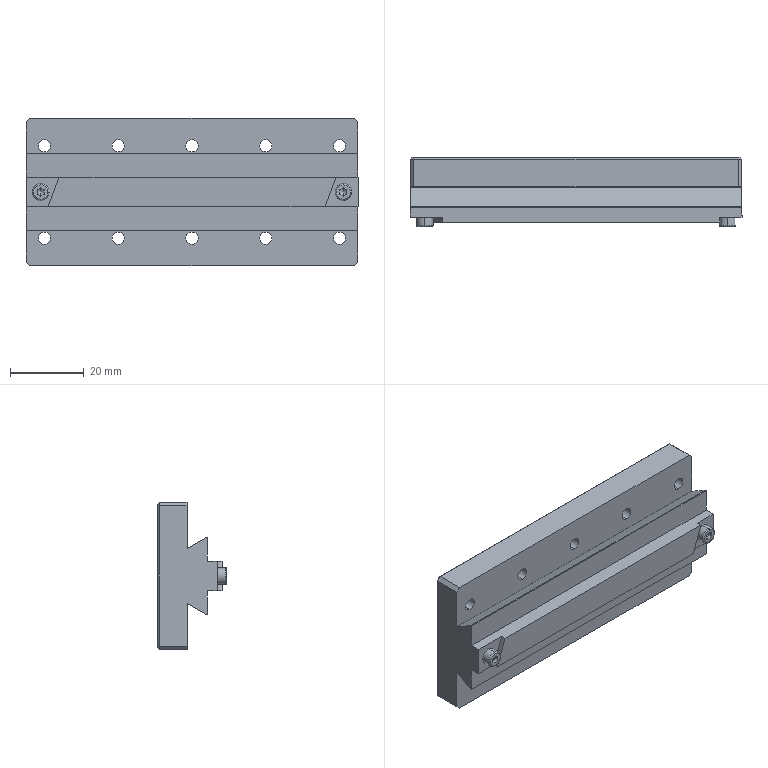Part | STEP file | Guide wheel mechanism revised.sldasm-Part-377 | 1 solid | 112 faces | box 90 x 18.7 x 40 mm | volume 39818 mm3 | plane 64 | cylinder 36 | cone 8 | torus 4 | commonest cylinder face diameters 3.3 x20 2.05 x4 2.5 x4 3 x4 4.5 x4